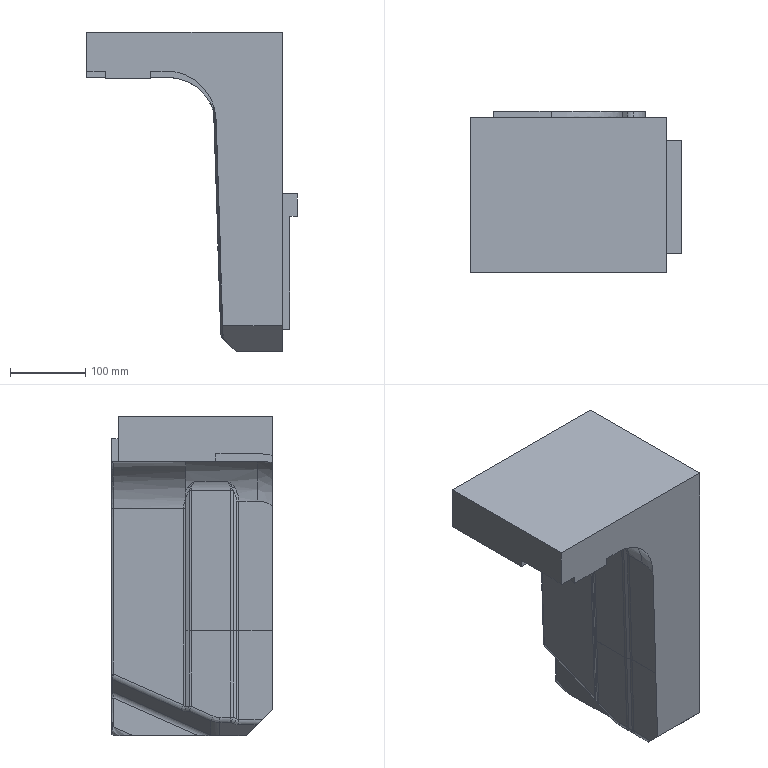Part | NX | features solid 2 | 1 solid | 100 faces | box 280 x 213.713 x 425 mm | volume 9892973 mm3 | plane 37 | spline 35 | cylinder 27 | sphere 1 | commonest cylinder face diameters 16 x7 20 x7 6 x4 200 x3 16.056 x2 130 x2